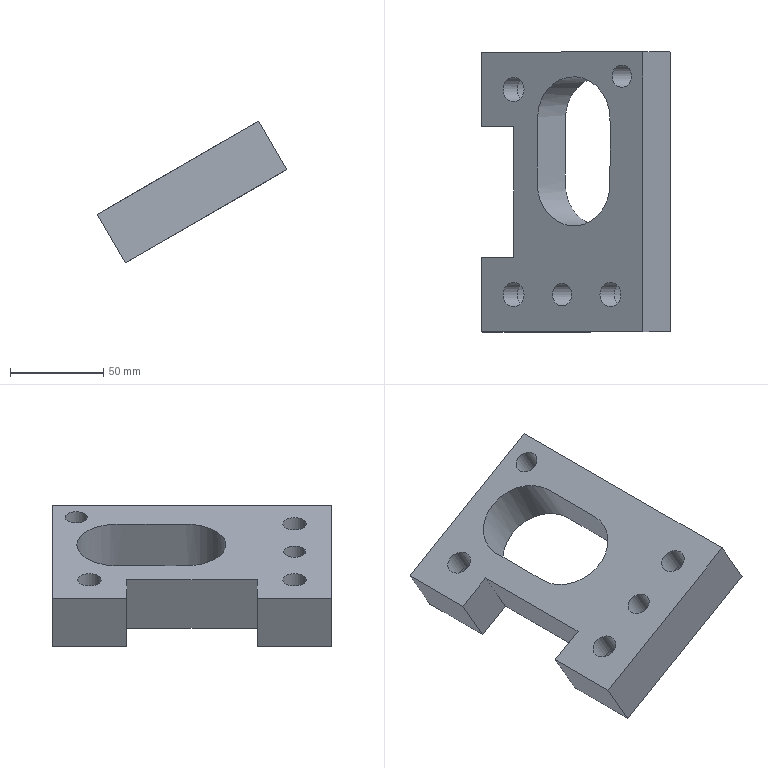Part | NX | features solid 2 | 1 solid | 22 faces | box 101.603 x 150 x 75.981 mm | volume 286509 mm3 | plane 13 | cylinder 8 | spline 1 | commonest cylinder face diameters 13 x3 20 x3 12 x2